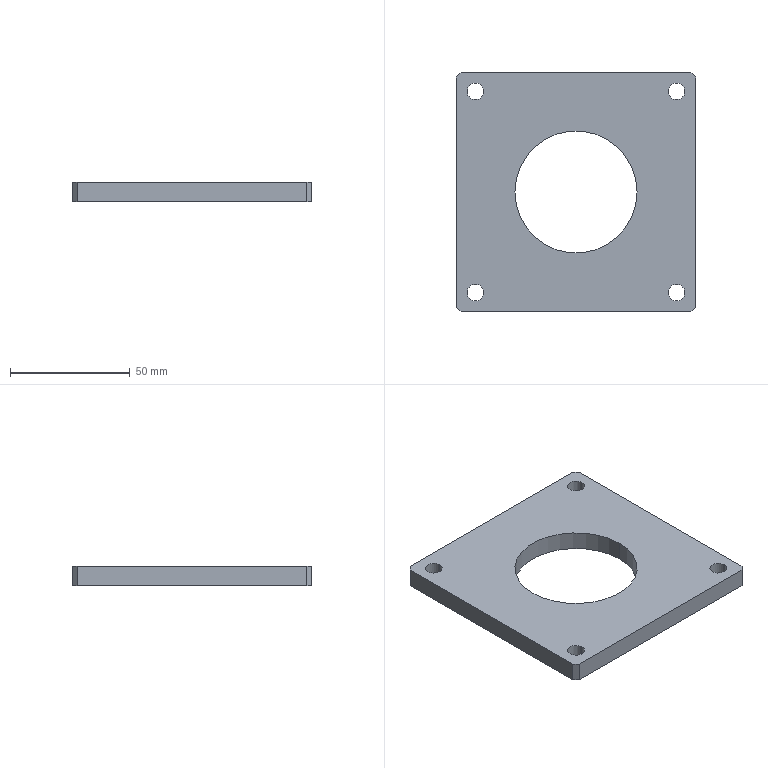Part | SolidWorks | features ICE 2, Chamfer 1, CirPattern 1, Extrusion 1 | 1 solid | 20 faces | box 100 x 100 x 8 mm | volume 62362 mm3 | cylinder 10 | plane 10 | commonest cylinder face diameters 7 x8 51 x2
STEP:
#1=CARTESIAN_POINT('',(-45.5,-42.,0.));
#2=VERTEX_POINT('',#1);
#3=CARTESIAN_POINT('',(-38.5,-42.,0.));
#4=VERTEX_POINT('',#3);
#5=CARTESIAN_POINT('',(-42.,-42.,0.));
#6=DIRECTION('',(0.,0.,1.));
#7=DIRECTION('',(-1.,0.,0.));
#8=AXIS2_PLACEMENT_3D('',#5,#6,#7);
#9=CIRCLE('',#8,3.5);
#10=EDGE_CURVE('',#2,#4,#9,.T.);
#11=ORIENTED_EDGE('',*,*,#10,.F.);
#12=CARTESIAN_POINT('',(-45.5,-42.,8.));
#13=VERTEX_POINT('',#12);
#14=CARTESIAN_POINT('',(-45.5,-42.,-0.001));
#15=DIRECTION('',(0.,0.,1.));
#16=VECTOR('',#15,1000.);
#17=LINE('',#14,#16);
#18=EDGE_CURVE('',#2,#13,#17,.T.);
#19=ORIENTED_EDGE('',*,*,#18,.T.);
#20=CARTESIAN_POINT('',(-38.5,-42.,8.));
#21=VERTEX_POINT('',#20);
#22=CARTESIAN_POINT('',(-42.,-42.,8.));
#23=DIRECTION('',(0.,0.,1.));
#24=DIRECTION('',(0.,1.,0.));
#25=AXIS2_PLACEMENT_3D('',#22,#23,#24);
#26=CIRCLE('',#25,3.5);
#27=EDGE_CURVE('',#13,#21,#26,.T.);
#28=ORIENTED_EDGE('',*,*,#27,.T.);
#29=CARTESIAN_POINT('',(-38.5,-42.,-0.001));
#30=DIRECTION('',(0.,0.,1.));
#31=VECTOR('',#30,1000.);
#32=LINE('',#29,#31);
#33=EDGE_CURVE('',#4,#21,#32,.T.);
#34=ORIENTED_EDGE('',*,*,#33,.F.);
#35=EDGE_LOOP('',(#11,#19,#28,#34));
#36=FACE_OUTER_BOUND('',#35,.T.);
#37=CARTESIAN_POINT('',(-42.,-42.,-0.001));
#38=DIRECTION('',(0.,0.,1.));
#39=DIRECTION('',(1.,0.,0.));
#40=AXIS2_PLACEMENT_3D('',#37,#38,#39);
#41=CYLINDRICAL_SURFACE('',#40,3.5);
#42=ADVANCED_FACE('',(#36),#41,.F.);
#43=CARTESIAN_POINT('',(38.5,-42.,0.));
#44=VERTEX_POINT('',#43);
#45=CARTESIAN_POINT('',(45.5,-42.,0.));
#46=VERTEX_POINT('',#45);
#47=CARTESIAN_POINT('',(42.,-42.,0.));
#48=DIRECTION('',(0.,0.,1.));
#49=DIRECTION('',(-1.,0.,0.));
#50=AXIS2_PLACEMENT_3D('',#47,#48,#49);
#51=CIRCLE('',#50,3.5);
#52=EDGE_CURVE('',#44,#46,#51,.T.);
#53=ORIENTED_EDGE('',*,*,#52,.F.);
#54=CARTESIAN_POINT('',(38.5,-42.,8.));
#55=VERTEX_POINT('',#54);
#56=CARTESIAN_POINT('',(38.5,-42.,-0.001));
#57=DIRECTION('',(0.,0.,1.));
#58=VECTOR('',#57,1000.);
#59=LINE('',#56,#58);
#60=EDGE_CURVE('',#44,#55,#59,.T.);
#61=ORIENTED_EDGE('',*,*,#60,.T.);
#62=CARTESIAN_POINT('',(45.5,-42.,8.));
#63=VERTEX_POINT('',#62);
#64=CARTESIAN_POINT('',(42.,-42.,8.));
#65=DIRECTION('',(0.,0.,1.));
#66=DIRECTION('',(-1.,0.,0.));
#67=AXIS2_PLACEMENT_3D('',#64,#65,#66);
#68=CIRCLE('',#67,3.5);
#69=EDGE_CURVE('',#55,#63,#68,.T.);
#70=ORIENTED_EDGE('',*,*,#69,.T.);
#71=CARTESIAN_POINT('',(45.5,-42.,-0.001));
#72=DIRECTION('',(0.,0.,1.));
#73=VECTOR('',#72,1000.);
#74=LINE('',#71,#73);
#75=EDGE_CURVE('',#46,#63,#74,.T.);
#76=ORIENTED_EDGE('',*,*,#75,.F.);
#77=EDGE_LOOP('',(#53,#61,#70,#76));
#78=FACE_OUTER_BOUND('',#77,.T.);
#79=CARTESIAN_POINT('',(42.,-42.,-0.001));
#80=DIRECTION('',(0.,0.,1.));
#81=DIRECTION('',(1.,0.,0.));
#82=AXIS2_PLACEMENT_3D('',#79,#80,#81);
#83=CYLINDRICAL_SURFACE('',#82,3.5);
#84=ADVANCED_FACE('',(#78),#83,.F.);
#85=CARTESIAN_POINT('',(38.5,42.,0.));
#86=VERTEX_POINT('',#85);
#87=CARTESIAN_POINT('',(45.5,42.,0.));
#88=VERTEX_POINT('',#87);
#89=CARTESIAN_POINT('',(42.,42.,0.));
#90=DIRECTION('',(0.,0.,1.));
#91=DIRECTION('',(-1.,0.,0.));
#92=AXIS2_PLACEMENT_3D('',#89,#90,#91);
#93=CIRCLE('',#92,3.5);
#94=EDGE_CURVE('',#86,#88,#93,.T.);
#95=ORIENTED_EDGE('',*,*,#94,.F.);
#96=CARTESIAN_POINT('',(38.5,42.,8.));
#97=VERTEX_POINT('',#96);
#98=CARTESIAN_POINT('',(38.5,42.,-0.001));
#99=DIRECTION('',(0.,0.,1.));
#100=VECTOR('',#99,1000.);
#101=LINE('',#98,#100);
#102=EDGE_CURVE('',#86,#97,#101,.T.);
#103=ORIENTED_EDGE('',*,*,#102,.T.);
#104=CARTESIAN_POINT('',(45.5,42.,8.));
#105=VERTEX_POINT('',#104);
#106=CARTESIAN_POINT('',(42.,42.,8.));
#107=DIRECTION('',(0.,0.,1.));
#108=DIRECTION('',(0.,-1.,0.));
#109=AXIS2_PLACEMENT_3D('',#106,#107,#108);
#110=CIRCLE('',#109,3.5);
#111=EDGE_CURVE('',#97,#105,#110,.T.);
#112=ORIENTED_EDGE('',*,*,#111,.T.);
#113=CARTESIAN_POINT('',(45.5,42.,-0.001));
#114=DIRECTION('',(0.,0.,1.));
#115=VECTOR('',#114,1000.);
#116=LINE('',#113,#115);
#117=EDGE_CURVE('',#88,#105,#116,.T.);
#118=ORIENTED_EDGE('',*,*,#117,.F.);
#119=EDGE_LOOP('',(#95,#103,#112,#118));
#120=FACE_OUTER_BOUND('',#119,.T.);
#121=CARTESIAN_POINT('',(42.,42.,-0.001));
#122=DIRECTION('',(0.,0.,1.));
#123=DIRECTION('',(1.,0.,0.));
#124=AXIS2_PLACEMENT_3D('',#121,#122,#123);
#125=CYLINDRICAL_SURFACE('',#124,3.5);
#126=ADVANCED_FACE('',(#120),#125,.F.);
#127=CARTESIAN_POINT('',(-45.5,42.,0.));
#128=VERTEX_POINT('',#127);
#129=CARTESIAN_POINT('',(-38.5,42.,0.));
#130=VERTEX_POINT('',#129);
#131=CARTESIAN_POINT('',(-42.,42.,0.));
#132=DIRECTION('',(0.,0.,1.));
#133=DIRECTION('',(-1.,0.,0.));
#134=AXIS2_PLACEMENT_3D('',#131,#132,#133);
#135=CIRCLE('',#134,3.5);
#136=EDGE_CURVE('',#128,#130,#135,.T.);
#137=ORIENTED_EDGE('',*,*,#136,.F.);
#138=CARTESIAN_POINT('',(-45.5,42.,8.));
#139=VERTEX_POINT('',#138);
#140=CARTESIAN_POINT('',(-45.5,42.,-0.001));
#141=DIRECTION('',(0.,0.,1.));
#142=VECTOR('',#141,1000.);
#143=LINE('',#140,#142);
#144=EDGE_CURVE('',#128,#139,#143,.T.);
#145=ORIENTED_EDGE('',*,*,#144,.T.);
#146=CARTESIAN_POINT('',(-38.5,42.,8.));
#147=VERTEX_POINT('',#146);
#148=CARTESIAN_POINT('',(-42.,42.,8.));
#149=DIRECTION('',(0.,0.,1.));
#150=DIRECTION('',(1.,0.,0.));
#151=AXIS2_PLACEMENT_3D('',#148,#149,#150);
#152=CIRCLE('',#151,3.5);
#153=EDGE_CURVE('',#139,#147,#152,.T.);
#154=ORIENTED_EDGE('',*,*,#153,.T.);
#155=CARTESIAN_POINT('',(-38.5,42.,-0.001));
#156=DIRECTION('',(0.,0.,1.));
#157=VECTOR('',#156,1000.);
#158=LINE('',#155,#157);
#159=EDGE_CURVE('',#130,#147,#158,.T.);
#160=ORIENTED_EDGE('',*,*,#159,.F.);
#161=EDGE_LOOP('',(#137,#145,#154,#160));
#162=FACE_OUTER_BOUND('',#161,.T.);
#163=CARTESIAN_POINT('',(-42.,42.,-0.001));
#164=DIRECTION('',(0.,0.,1.));
#165=DIRECTION('',(1.,0.,0.));
#166=AXIS2_PLACEMENT_3D('',#163,#164,#165);
#167=CYLINDRICAL_SURFACE('',#166,3.5);
#168=ADVANCED_FACE('',(#162),#167,.F.);
#169=CARTESIAN_POINT('',(-25.5,0.,0.));
#170=VERTEX_POINT('',#169);
#171=CARTESIAN_POINT('',(25.5,0.,0.));
#172=VERTEX_POINT('',#171);
#173=CARTESIAN_POINT('',(0.,0.,0.));
#174=DIRECTION('',(0.,0.,1.));
#175=DIRECTION('',(-1.,0.,0.));
#176=AXIS2_PLACEMENT_3D('',#173,#174,#175);
#177=CIRCLE('',#176,25.5);
#178=EDGE_CURVE('',#170,#172,#177,.T.);
#179=ORIENTED_EDGE('',*,*,#178,.F.);
#180=CARTESIAN_POINT('',(-25.5,0.,8.));
#181=VERTEX_POINT('',#180);
#182=CARTESIAN_POINT('',(-25.5,0.,-0.001));
#183=DIRECTION('',(0.,0.,1.));
#184=VECTOR('',#183,1000.);
#185=LINE('',#182,#184);
#186=EDGE_CURVE('',#170,#181,#185,.T.);
#187=ORIENTED_EDGE('',*,*,#186,.T.);
#188=CARTESIAN_POINT('',(25.5,0.,8.));
#189=VERTEX_POINT('',#188);
#190=CARTESIAN_POINT('',(0.,0.,8.));
#191=DIRECTION('',(0.,0.,1.));
#192=DIRECTION('',(1.,0.,0.));
#193=AXIS2_PLACEMENT_3D('',#190,#191,#192);
#194=CIRCLE('',#193,25.5);
#195=EDGE_CURVE('',#181,#189,#194,.T.);
#196=ORIENTED_EDGE('',*,*,#195,.T.);
#197=CARTESIAN_POINT('',(25.5,0.,-0.001));
#198=DIRECTION('',(0.,0.,1.));
#199=VECTOR('',#198,1000.);
#200=LINE('',#197,#199);
#201=EDGE_CURVE('',#172,#189,#200,.T.);
#202=ORIENTED_EDGE('',*,*,#201,.F.);
#203=EDGE_LOOP('',(#179,#187,#196,#202));
#204=FACE_OUTER_BOUND('',#203,.T.);
#205=CARTESIAN_POINT('',(0.,0.,-0.001));
#206=DIRECTION('',(0.,0.,1.));
#207=DIRECTION('',(1.,0.,0.));
#208=AXIS2_PLACEMENT_3D('',#205,#206,#207);
#209=CYLINDRICAL_SURFACE('',#208,25.5);
#210=ADVANCED_FACE('',(#204),#209,.F.);
#211=CARTESIAN_POINT('',(50.,-48.,0.));
#212=VERTEX_POINT('',#211);
#213=CARTESIAN_POINT('',(50.,48.,0.));
#214=VERTEX_POINT('',#213);
#215=CARTESIAN_POINT('',(50.,-50.,0.));
#216=DIRECTION('',(0.,1.,0.));
#217=VECTOR('',#216,1000.);
#218=LINE('',#215,#217);
#219=EDGE_CURVE('',#212,#214,#218,.T.);
#220=ORIENTED_EDGE('',*,*,#219,.T.);
#221=CARTESIAN_POINT('',(50.,48.,8.));
#222=VERTEX_POINT('',#221);
#223=CARTESIAN_POINT('',(50.,48.,8.));
#224=DIRECTION('',(0.,0.,1.));
#225=VECTOR('',#224,1000.);
#226=LINE('',#223,#225);
#227=EDGE_CURVE('',#214,#222,#226,.T.);
#228=ORIENTED_EDGE('',*,*,#227,.T.);
#229=CARTESIAN_POINT('',(50.,-48.,8.));
#230=VERTEX_POINT('',#229);
#231=CARTESIAN_POINT('',(50.,-50.,8.));
#232=DIRECTION('',(0.,1.,0.));
#233=VECTOR('',#232,1000.);
#234=LINE('',#231,#233);
#235=EDGE_CURVE('',#230,#222,#234,.T.);
#236=ORIENTED_EDGE('',*,*,#235,.F.);
#237=CARTESIAN_POINT('',(50.,-48.,8.));
#238=DIRECTION('',(0.,0.,-1.));
#239=VECTOR('',#238,1000.);
#240=LINE('',#237,#239);
#241=EDGE_CURVE('',#230,#212,#240,.T.);
#242=ORIENTED_EDGE('',*,*,#241,.T.);
#243=EDGE_LOOP('',(#220,#228,#236,#242));
#244=FACE_OUTER_BOUND('',#243,.T.);
#245=CARTESIAN_POINT('',(50.,-50.,8.));
#246=DIRECTION('',(-1.,0.,0.));
#247=DIRECTION('',(0.,0.,1.));
#248=AXIS2_PLACEMENT_3D('',#245,#246,#247);
#249=PLANE('',#248);
#250=ADVANCED_FACE('',(#244),#249,.F.);
#251=CARTESIAN_POINT('',(48.,50.,8.));
#252=VERTEX_POINT('',#251);
#253=CARTESIAN_POINT('',(-48.,50.,8.));
#254=VERTEX_POINT('',#253);
#255=CARTESIAN_POINT('',(-50.,50.,8.));
#256=DIRECTION('',(-1.,0.,0.));
#257=VECTOR('',#256,1000.);
#258=LINE('',#255,#257);
#259=EDGE_CURVE('',#252,#254,#258,.T.);
#260=ORIENTED_EDGE('',*,*,#259,.F.);
#261=CARTESIAN_POINT('',(48.,50.,0.));
#262=VERTEX_POINT('',#261);
#263=CARTESIAN_POINT('',(48.,50.,8.));
#264=DIRECTION('',(0.,0.,-1.));
#265=VECTOR('',#264,1000.);
#266=LINE('',#263,#265);
#267=EDGE_CURVE('',#252,#262,#266,.T.);
#268=ORIENTED_EDGE('',*,*,#267,.T.);
#269=CARTESIAN_POINT('',(-48.,50.,0.));
#270=VERTEX_POINT('',#269);
#271=CARTESIAN_POINT('',(-50.,50.,0.));
#272=DIRECTION('',(-1.,0.,0.));
#273=VECTOR('',#272,1000.);
#274=LINE('',#271,#273);
#275=EDGE_CURVE('',#262,#270,#274,.T.);
#276=ORIENTED_EDGE('',*,*,#275,.T.);
#277=CARTESIAN_POINT('',(-48.,50.,8.));
#278=DIRECTION('',(0.,0.,1.));
#279=VECTOR('',#278,1000.);
#280=LINE('',#277,#279);
#281=EDGE_CURVE('',#270,#254,#280,.T.);
#282=ORIENTED_EDGE('',*,*,#281,.T.);
#283=EDGE_LOOP('',(#260,#268,#276,#282));
#284=FACE_OUTER_BOUND('',#283,.T.);
#285=CARTESIAN_POINT('',(-50.,50.,8.));
#286=DIRECTION('',(0.,-1.,0.));
#287=DIRECTION('',(0.,0.,-1.));
#288=AXIS2_PLACEMENT_3D('',#285,#286,#287);
#289=PLANE('',#288);
#290=ADVANCED_FACE('',(#284),#289,.F.);
#291=CARTESIAN_POINT('',(-50.,48.,8.));
#292=VERTEX_POINT('',#291);
#293=CARTESIAN_POINT('',(-50.,-48.,8.));
#294=VERTEX_POINT('',#293);
#295=CARTESIAN_POINT('',(-50.,-50.,8.));
#296=DIRECTION('',(0.,-1.,0.));
#297=VECTOR('',#296,1000.);
#298=LINE('',#295,#297);
#299=EDGE_CURVE('',#292,#294,#298,.T.);
#300=ORIENTED_EDGE('',*,*,#299,.F.);
#301=CARTESIAN_POINT('',(-50.,48.,0.));
#302=VERTEX_POINT('',#301);
#303=CARTESIAN_POINT('',(-50.,48.,8.));
#304=DIRECTION('',(0.,0.,-1.));
#305=VECTOR('',#304,1000.);
#306=LINE('',#303,#305);
#307=EDGE_CURVE('',#292,#302,#306,.T.);
#308=ORIENTED_EDGE('',*,*,#307,.T.);
#309=CARTESIAN_POINT('',(-50.,-48.,0.));
#310=VERTEX_POINT('',#309);
#311=CARTESIAN_POINT('',(-50.,-50.,0.));
#312=DIRECTION('',(0.,-1.,0.));
#313=VECTOR('',#312,1000.);
#314=LINE('',#311,#313);
#315=EDGE_CURVE('',#302,#310,#314,.T.);
#316=ORIENTED_EDGE('',*,*,#315,.T.);
#317=CARTESIAN_POINT('',(-50.,-48.,8.));
#318=DIRECTION('',(0.,0.,1.));
#319=VECTOR('',#318,1000.);
#320=LINE('',#317,#319);
#321=EDGE_CURVE('',#310,#294,#320,.T.);
#322=ORIENTED_EDGE('',*,*,#321,.T.);
#323=EDGE_LOOP('',(#300,#308,#316,#322));
#324=FACE_OUTER_BOUND('',#323,.T.);
#325=CARTESIAN_POINT('',(-50.,-50.,8.));
#326=DIRECTION('',(1.,0.,0.));
#327=DIRECTION('',(0.,0.,-1.));
#328=AXIS2_PLACEMENT_3D('',#325,#326,#327);
#329=PLANE('',#328);
#330=ADVANCED_FACE('',(#324),#329,.F.);
#331=CARTESIAN_POINT('',(-48.,-50.,0.));
#332=VERTEX_POINT('',#331);
#333=CARTESIAN_POINT('',(48.,-50.,0.));
#334=VERTEX_POINT('',#333);
#335=CARTESIAN_POINT('',(-50.,-50.,0.));
#336=DIRECTION('',(1.,0.,0.));
#337=VECTOR('',#336,1000.);
#338=LINE('',#335,#337);
#339=EDGE_CURVE('',#332,#334,#338,.T.);
#340=ORIENTED_EDGE('',*,*,#339,.T.);
#341=CARTESIAN_POINT('',(48.,-50.,8.));
#342=VERTEX_POINT('',#341);
#343=CARTESIAN_POINT('',(48.,-50.,8.));
#344=DIRECTION('',(0.,0.,1.));
#345=VECTOR('',#344,1000.);
#346=LINE('',#343,#345);
#347=EDGE_CURVE('',#334,#342,#346,.T.);
#348=ORIENTED_EDGE('',*,*,#347,.T.);
#349=CARTESIAN_POINT('',(-48.,-50.,8.));
#350=VERTEX_POINT('',#349);
#351=CARTESIAN_POINT('',(-50.,-50.,8.));
#352=DIRECTION('',(1.,0.,0.));
#353=VECTOR('',#352,1000.);
#354=LINE('',#351,#353);
#355=EDGE_CURVE('',#350,#342,#354,.T.);
#356=ORIENTED_EDGE('',*,*,#355,.F.);
#357=CARTESIAN_POINT('',(-48.,-50.,8.));
#358=DIRECTION('',(0.,0.,-1.));
#359=VECTOR('',#358,1000.);
#360=LINE('',#357,#359);
#361=EDGE_CURVE('',#350,#332,#360,.T.);
#362=ORIENTED_EDGE('',*,*,#361,.T.);
#363=EDGE_LOOP('',(#340,#348,#356,#362));
#364=FACE_OUTER_BOUND('',#363,.T.);
#365=CARTESIAN_POINT('',(-50.,-50.,8.));
#366=DIRECTION('',(0.,1.,0.));
#367=DIRECTION('',(0.,0.,1.));
#368=AXIS2_PLACEMENT_3D('',#365,#366,#367);
#369=PLANE('',#368);
#370=ADVANCED_FACE('',(#364),#369,.F.);
#371=CARTESIAN_POINT('',(-42.,-42.,8.));
#372=DIRECTION('',(0.,0.,1.));
#373=DIRECTION('',(0.,1.,0.));
#374=AXIS2_PLACEMENT_3D('',#371,#372,#373);
#375=CIRCLE('',#374,3.5);
#376=EDGE_CURVE('',#21,#13,#375,.T.);
#377=ORIENTED_EDGE('',*,*,#376,.F.);
#378=ORIENTED_EDGE('',*,*,#27,.F.);
#379=EDGE_LOOP('',(#377,#378));
#380=FACE_BOUND('',#379,.T.);
#381=CARTESIAN_POINT('',(42.,-42.,8.));
#382=DIRECTION('',(0.,0.,1.));
#383=DIRECTION('',(-1.,0.,0.));
#384=AXIS2_PLACEMENT_3D('',#381,#382,#383);
#385=CIRCLE('',#384,3.5);
#386=EDGE_CURVE('',#63,#55,#385,.T.);
#387=ORIENTED_EDGE('',*,*,#386,.F.);
#388=ORIENTED_EDGE('',*,*,#69,.F.);
#389=EDGE_LOOP('',(#387,#388));
#390=FACE_BOUND('',#389,.T.);
#391=CARTESIAN_POINT('',(42.,42.,8.));
#392=DIRECTION('',(0.,0.,1.));
#393=DIRECTION('',(0.,-1.,0.));
#394=AXIS2_PLACEMENT_3D('',#391,#392,#393);
#395=CIRCLE('',#394,3.5);
#396=EDGE_CURVE('',#105,#97,#395,.T.);
#397=ORIENTED_EDGE('',*,*,#396,.F.);
#398=ORIENTED_EDGE('',*,*,#111,.F.);
#399=EDGE_LOOP('',(#397,#398));
#400=FACE_BOUND('',#399,.T.);
#401=CARTESIAN_POINT('',(-42.,42.,8.));
#402=DIRECTION('',(0.,0.,1.));
#403=DIRECTION('',(1.,0.,0.));
#404=AXIS2_PLACEMENT_3D('',#401,#402,#403);
#405=CIRCLE('',#404,3.5);
#406=EDGE_CURVE('',#147,#139,#405,.T.);
#407=ORIENTED_EDGE('',*,*,#406,.F.);
#408=ORIENTED_EDGE('',*,*,#153,.F.);
#409=EDGE_LOOP('',(#407,#408));
#410=FACE_BOUND('',#409,.T.);
#411=CARTESIAN_POINT('',(0.,0.,8.));
#412=DIRECTION('',(0.,0.,1.));
#413=DIRECTION('',(1.,0.,0.));
#414=AXIS2_PLACEMENT_3D('',#411,#412,#413);
#415=CIRCLE('',#414,25.5);
#416=EDGE_CURVE('',#189,#181,#415,.T.);
#417=ORIENTED_EDGE('',*,*,#416,.F.);
#418=ORIENTED_EDGE('',*,*,#195,.F.);
#419=EDGE_LOOP('',(#417,#418));
#420=FACE_BOUND('',#419,.T.);
#421=ORIENTED_EDGE('',*,*,#235,.T.);
#422=CARTESIAN_POINT('',(48.,50.,8.));
#423=DIRECTION('',(-0.7071,0.7071,0.));
#424=VECTOR('',#423,1000.);
#425=LINE('',#422,#424);
#426=EDGE_CURVE('',#222,#252,#425,.T.);
#427=ORIENTED_EDGE('',*,*,#426,.T.);
#428=ORIENTED_EDGE('',*,*,#259,.T.);
#429=CARTESIAN_POINT('',(-50.,48.,8.));
#430=DIRECTION('',(-0.7071,-0.7071,0.));
#431=VECTOR('',#430,1000.);
#432=LINE('',#429,#431);
#433=EDGE_CURVE('',#254,#292,#432,.T.);
#434=ORIENTED_EDGE('',*,*,#433,.T.);
#435=ORIENTED_EDGE('',*,*,#299,.T.);
#436=CARTESIAN_POINT('',(-48.,-50.,8.));
#437=DIRECTION('',(0.7071,-0.7071,0.));
#438=VECTOR('',#437,1000.);
#439=LINE('',#436,#438);
#440=EDGE_CURVE('',#294,#350,#439,.T.);
#441=ORIENTED_EDGE('',*,*,#440,.T.);
#442=ORIENTED_EDGE('',*,*,#355,.T.);
#443=CARTESIAN_POINT('',(50.,-48.,8.));
#444=DIRECTION('',(0.7071,0.7071,0.));
#445=VECTOR('',#444,1000.);
#446=LINE('',#443,#445);
#447=EDGE_CURVE('',#342,#230,#446,.T.);
#448=ORIENTED_EDGE('',*,*,#447,.T.);
#449=EDGE_LOOP('',(#421,#427,#428,#434,#435,#441,#442,#448));
#450=FACE_OUTER_BOUND('',#449,.T.);
#451=CARTESIAN_POINT('',(0.,0.,8.));
#452=DIRECTION('',(0.,0.,-1.));
#453=DIRECTION('',(-1.,0.,0.));
#454=AXIS2_PLACEMENT_3D('',#451,#452,#453);
#455=PLANE('',#454);
#456=ADVANCED_FACE('',(#380,#390,#400,#410,#420,#450),#455,.F.);
#457=CARTESIAN_POINT('',(-42.,-42.,0.));
#458=DIRECTION('',(0.,0.,1.));
#459=DIRECTION('',(-1.,0.,0.));
#460=AXIS2_PLACEMENT_3D('',#457,#458,#459);
#461=CIRCLE('',#460,3.5);
#462=EDGE_CURVE('',#4,#2,#461,.T.);
#463=ORIENTED_EDGE('',*,*,#462,.T.);
#464=ORIENTED_EDGE('',*,*,#10,.T.);
#465=EDGE_LOOP('',(#463,#464));
#466=FACE_BOUND('',#465,.T.);
#467=CARTESIAN_POINT('',(42.,-42.,0.));
#468=DIRECTION('',(0.,0.,1.));
#469=DIRECTION('',(-1.,0.,0.));
#470=AXIS2_PLACEMENT_3D('',#467,#468,#469);
#471=CIRCLE('',#470,3.5);
#472=EDGE_CURVE('',#46,#44,#471,.T.);
#473=ORIENTED_EDGE('',*,*,#472,.T.);
#474=ORIENTED_EDGE('',*,*,#52,.T.);
#475=EDGE_LOOP('',(#473,#474));
#476=FACE_BOUND('',#475,.T.);
#477=CARTESIAN_POINT('',(42.,42.,0.));
#478=DIRECTION('',(0.,0.,1.));
#479=DIRECTION('',(-1.,0.,0.));
#480=AXIS2_PLACEMENT_3D('',#477,#478,#479);
#481=CIRCLE('',#480,3.5);
#482=EDGE_CURVE('',#88,#86,#481,.T.);
#483=ORIENTED_EDGE('',*,*,#482,.T.);
#484=ORIENTED_EDGE('',*,*,#94,.T.);
#485=EDGE_LOOP('',(#483,#484));
#486=FACE_BOUND('',#485,.T.);
#487=CARTESIAN_POINT('',(-42.,42.,0.));
#488=DIRECTION('',(0.,0.,1.));
#489=DIRECTION('',(-1.,0.,0.));
#490=AXIS2_PLACEMENT_3D('',#487,#488,#489);
#491=CIRCLE('',#490,3.5);
#492=EDGE_CURVE('',#130,#128,#491,.T.);
#493=ORIENTED_EDGE('',*,*,#492,.T.);
#494=ORIENTED_EDGE('',*,*,#136,.T.);
#495=EDGE_LOOP('',(#493,#494));
#496=FACE_BOUND('',#495,.T.);
#497=CARTESIAN_POINT('',(0.,0.,0.));
#498=DIRECTION('',(0.,0.,1.));
#499=DIRECTION('',(-1.,0.,0.));
#500=AXIS2_PLACEMENT_3D('',#497,#498,#499);
#501=CIRCLE('',#500,25.5);
#502=EDGE_CURVE('',#172,#170,#501,.T.);
#503=ORIENTED_EDGE('',*,*,#502,.T.);
#504=ORIENTED_EDGE('',*,*,#178,.T.);
#505=EDGE_LOOP('',(#503,#504));
#506=FACE_BOUND('',#505,.T.);
#507=ORIENTED_EDGE('',*,*,#275,.F.);
#508=CARTESIAN_POINT('',(49.,49.,0.));
#509=DIRECTION('',(0.7071,-0.7071,0.));
#510=VECTOR('',#509,1000.);
#511=LINE('',#508,#510);
#512=EDGE_CURVE('',#262,#214,#511,.T.);
#513=ORIENTED_EDGE('',*,*,#512,.T.);
#514=ORIENTED_EDGE('',*,*,#219,.F.);
#515=CARTESIAN_POINT('',(49.,-49.,0.));
#516=DIRECTION('',(-0.7071,-0.7071,0.));
#517=VECTOR('',#516,1000.);
#518=LINE('',#515,#517);
#519=EDGE_CURVE('',#212,#334,#518,.T.);
#520=ORIENTED_EDGE('',*,*,#519,.T.);
#521=ORIENTED_EDGE('',*,*,#339,.F.);
#522=CARTESIAN_POINT('',(-49.,-49.,0.));
#523=DIRECTION('',(-0.7071,0.7071,0.));
#524=VECTOR('',#523,1000.);
#525=LINE('',#522,#524);
#526=EDGE_CURVE('',#332,#310,#525,.T.);
#527=ORIENTED_EDGE('',*,*,#526,.T.);
#528=ORIENTED_EDGE('',*,*,#315,.F.);
#529=CARTESIAN_POINT('',(-49.,49.,0.));
#530=DIRECTION('',(0.7071,0.7071,0.));
#531=VECTOR('',#530,1000.);
#532=LINE('',#529,#531);
#533=EDGE_CURVE('',#302,#270,#532,.T.);
#534=ORIENTED_EDGE('',*,*,#533,.T.);
#535=EDGE_LOOP('',(#507,#513,#514,#520,#521,#527,#528,#534));
#536=FACE_OUTER_BOUND('',#535,.T.);
#537=CARTESIAN_POINT('',(0.,0.,0.));
#538=DIRECTION('',(0.,0.,-1.));
#539=DIRECTION('',(-1.,0.,0.));
#540=AXIS2_PLACEMENT_3D('',#537,#538,#539);
#541=PLANE('',#540);
#542=ADVANCED_FACE('',(#466,#476,#486,#496,#506,#536),#541,.T.);
#543=ORIENTED_EDGE('',*,*,#186,.F.);
#544=ORIENTED_EDGE('',*,*,#502,.F.);
#545=ORIENTED_EDGE('',*,*,#201,.T.);
#546=ORIENTED_EDGE('',*,*,#416,.T.);
#547=EDGE_LOOP('',(#543,#544,#545,#546));
#548=FACE_OUTER_BOUND('',#547,.T.);
#549=CARTESIAN_POINT('',(0.,0.,-0.001));
#550=DIRECTION('',(0.,0.,1.));
#551=DIRECTION('',(1.,0.,0.));
#552=AXIS2_PLACEMENT_3D('',#549,#550,#551);
#553=CYLINDRICAL_SURFACE('',#552,25.5);
#554=ADVANCED_FACE('',(#548),#553,.F.);
#555=ORIENTED_EDGE('',*,*,#144,.F.);
#556=ORIENTED_EDGE('',*,*,#492,.F.);
#557=ORIENTED_EDGE('',*,*,#159,.T.);
#558=ORIENTED_EDGE('',*,*,#406,.T.);
#559=EDGE_LOOP('',(#555,#556,#557,#558));
#560=FACE_OUTER_BOUND('',#559,.T.);
#561=CARTESIAN_POINT('',(-42.,42.,-0.001));
#562=DIRECTION('',(0.,0.,1.));
#563=DIRECTION('',(1.,0.,0.));
#564=AXIS2_PLACEMENT_3D('',#561,#562,#563);
#565=CYLINDRICAL_SURFACE('',#564,3.5);
#566=ADVANCED_FACE('',(#560),#565,.F.);
#567=ORIENTED_EDGE('',*,*,#102,.F.);
#568=ORIENTED_EDGE('',*,*,#482,.F.);
#569=ORIENTED_EDGE('',*,*,#117,.T.);
#570=ORIENTED_EDGE('',*,*,#396,.T.);
#571=EDGE_LOOP('',(#567,#568,#569,#570));
#572=FACE_OUTER_BOUND('',#571,.T.);
#573=CARTESIAN_POINT('',(42.,42.,-0.001));
#574=DIRECTION('',(0.,0.,1.));
#575=DIRECTION('',(1.,0.,0.));
#576=AXIS2_PLACEMENT_3D('',#573,#574,#575);
#577=CYLINDRICAL_SURFACE('',#576,3.5);
#578=ADVANCED_FACE('',(#572),#577,.F.);
#579=ORIENTED_EDGE('',*,*,#60,.F.);
#580=ORIENTED_EDGE('',*,*,#472,.F.);
#581=ORIENTED_EDGE('',*,*,#75,.T.);
#582=ORIENTED_EDGE('',*,*,#386,.T.);
#583=EDGE_LOOP('',(#579,#580,#581,#582));
#584=FACE_OUTER_BOUND('',#583,.T.);
#585=CARTESIAN_POINT('',(42.,-42.,-0.001));
#586=DIRECTION('',(0.,0.,1.));
#587=DIRECTION('',(1.,0.,0.));
#588=AXIS2_PLACEMENT_3D('',#585,#586,#587);
#589=CYLINDRICAL_SURFACE('',#588,3.5);
#590=ADVANCED_FACE('',(#584),#589,.F.);
#591=ORIENTED_EDGE('',*,*,#18,.F.);
#592=ORIENTED_EDGE('',*,*,#462,.F.);
#593=ORIENTED_EDGE('',*,*,#33,.T.);
#594=ORIENTED_EDGE('',*,*,#376,.T.);
#595=EDGE_LOOP('',(#591,#592,#593,#594));
#596=FACE_OUTER_BOUND('',#595,.T.);
#597=CARTESIAN_POINT('',(-42.,-42.,-0.001));
#598=DIRECTION('',(0.,0.,1.));
#599=DIRECTION('',(1.,0.,0.));
#600=AXIS2_PLACEMENT_3D('',#597,#598,#599);
#601=CYLINDRICAL_SURFACE('',#600,3.5);
#602=ADVANCED_FACE('',(#596),#601,.F.);
#603=ORIENTED_EDGE('',*,*,#426,.F.);
#604=ORIENTED_EDGE('',*,*,#227,.F.);
#605=ORIENTED_EDGE('',*,*,#512,.F.);
#606=ORIENTED_EDGE('',*,*,#267,.F.);
#607=EDGE_LOOP('',(#603,#604,#605,#606));
#608=FACE_OUTER_BOUND('',#607,.T.);
#609=CARTESIAN_POINT('',(48.,50.,8.));
#610=DIRECTION('',(-0.7071,-0.7071,0.));
#611=DIRECTION('',(0.,0.,-1.));
#612=AXIS2_PLACEMENT_3D('',#609,#610,#611);
#613=PLANE('',#612);
#614=ADVANCED_FACE('',(#608),#613,.F.);
#615=ORIENTED_EDGE('',*,*,#433,.F.);
#616=ORIENTED_EDGE('',*,*,#281,.F.);
#617=ORIENTED_EDGE('',*,*,#533,.F.);
#618=ORIENTED_EDGE('',*,*,#307,.F.);
#619=EDGE_LOOP('',(#615,#616,#617,#618));
#620=FACE_OUTER_BOUND('',#619,.T.);
#621=CARTESIAN_POINT('',(-50.,48.,8.));
#622=DIRECTION('',(0.7071,-0.7071,0.));
#623=DIRECTION('',(0.,0.,-1.));
#624=AXIS2_PLACEMENT_3D('',#621,#622,#623);
#625=PLANE('',#624);
#626=ADVANCED_FACE('',(#620),#625,.F.);
#627=ORIENTED_EDGE('',*,*,#447,.F.);
#628=ORIENTED_EDGE('',*,*,#347,.F.);
#629=ORIENTED_EDGE('',*,*,#519,.F.);
#630=ORIENTED_EDGE('',*,*,#241,.F.);
#631=EDGE_LOOP('',(#627,#628,#629,#630));
#632=FACE_OUTER_BOUND('',#631,.T.);
#633=CARTESIAN_POINT('',(50.,-48.,8.));
#634=DIRECTION('',(-0.7071,0.7071,0.));
#635=DIRECTION('',(0.,0.,-1.));
#636=AXIS2_PLACEMENT_3D('',#633,#634,#635);
#637=PLANE('',#636);
#638=ADVANCED_FACE('',(#632),#637,.F.);
#639=ORIENTED_EDGE('',*,*,#440,.F.);
#640=ORIENTED_EDGE('',*,*,#321,.F.);
#641=ORIENTED_EDGE('',*,*,#526,.F.);
#642=ORIENTED_EDGE('',*,*,#361,.F.);
#643=EDGE_LOOP('',(#639,#640,#641,#642));
#644=FACE_OUTER_BOUND('',#643,.T.);
#645=CARTESIAN_POINT('',(-48.,-50.,8.));
#646=DIRECTION('',(0.7071,0.7071,0.));
#647=DIRECTION('',(0.,0.,-1.));
#648=AXIS2_PLACEMENT_3D('',#645,#646,#647);
#649=PLANE('',#648);
#650=ADVANCED_FACE('',(#644),#649,.F.);
#651=CLOSED_SHELL('',(#42,#84,#126,#168,#210,#250,#290,#330,#370,#456,#542,#554,#566,#578,#590,#602,#614,#626,#638,#650));
#652=MANIFOLD_SOLID_BREP('',#651);
#653=CARTESIAN_POINT('',(0.,0.,0.));
#654=DIRECTION('',(0.,0.,1.));
#655=DIRECTION('',(1.,0.,0.));
#656=AXIS2_PLACEMENT_3D('',#653,#654,#655);
#657=(LENGTH_UNIT()NAMED_UNIT(*)SI_UNIT(.MILLI.,.METRE.));
#658=UNCERTAINTY_MEASURE_WITH_UNIT(LENGTH_MEASURE(0.00001),#657,'','');
#659=(NAMED_UNIT(*)PLANE_ANGLE_UNIT()SI_UNIT($,.RADIAN.));
#660=(NAMED_UNIT(*)SI_UNIT($,.STERADIAN.)SOLID_ANGLE_UNIT());
#661=(GEOMETRIC_REPRESENTATION_CONTEXT(3)GLOBAL_UNCERTAINTY_ASSIGNED_CONTEXT((#658))GLOBAL_UNIT_ASSIGNED_CONTEXT((#657,#659,#660))REPRESENTATION_CONTEXT('',''));
#662=ADVANCED_BREP_SHAPE_REPRESENTATION('',(#652,#656),#661);